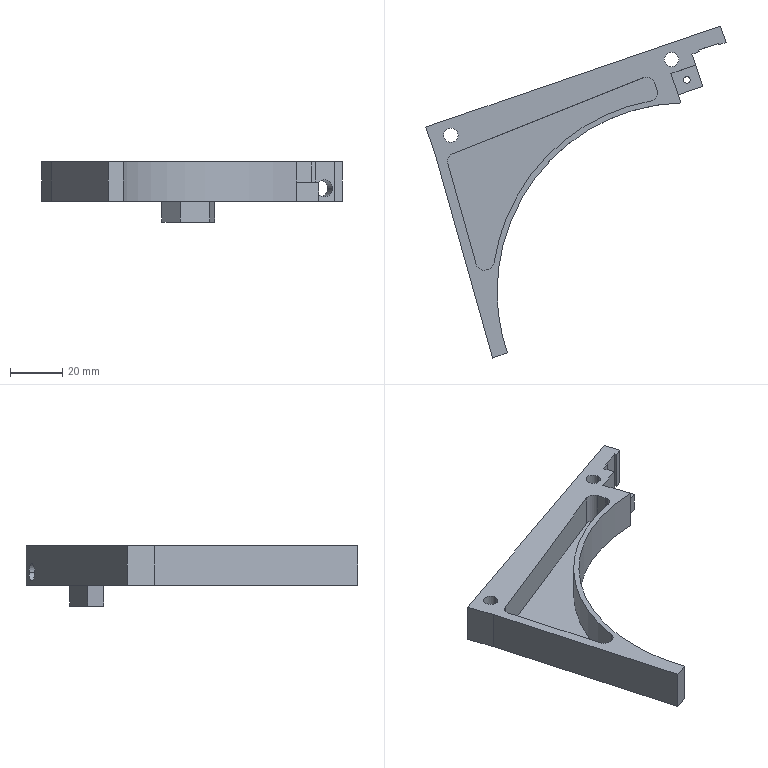Part | SolidWorks | features Cut 4, HoleWzd 2, Extrusion 1, ICE 1 | 1 solid | 45 faces | box 114.513 x 126.581 x 23 mm | volume 34516 mm3 | plane 28 | cylinder 17 | commonest cylinder face diameters 6 x6 5.5 x4 2.5 x2 6.5 x2 144 x2 148 x1
STEP:
#1=CARTESIAN_POINT('',(227.407,180.394,0.));
#2=VERTEX_POINT('',#1);
#3=CARTESIAN_POINT('',(229.907,180.394,0.));
#4=VERTEX_POINT('',#3);
#5=CARTESIAN_POINT('',(228.657,180.394,0.));
#6=DIRECTION('',(0.,0.,1.));
#7=DIRECTION('',(1.,0.,0.));
#8=AXIS2_PLACEMENT_3D('',#5,#6,#7);
#9=CIRCLE('',#8,1.25);
#10=EDGE_CURVE('',#2,#4,#9,.T.);
#11=ORIENTED_EDGE('',*,*,#10,.F.);
#12=CARTESIAN_POINT('',(227.407,180.394,7.));
#13=VERTEX_POINT('',#12);
#14=CARTESIAN_POINT('',(227.407,180.394,7.));
#15=DIRECTION('',(0.,0.,1.));
#16=VECTOR('',#15,1000.);
#17=LINE('',#14,#16);
#18=EDGE_CURVE('',#2,#13,#17,.T.);
#19=ORIENTED_EDGE('',*,*,#18,.T.);
#20=CARTESIAN_POINT('',(229.907,180.394,7.));
#21=VERTEX_POINT('',#20);
#22=CARTESIAN_POINT('',(228.657,180.394,7.));
#23=DIRECTION('',(0.,0.,1.));
#24=DIRECTION('',(1.,0.,0.));
#25=AXIS2_PLACEMENT_3D('',#22,#23,#24);
#26=CIRCLE('',#25,1.25);
#27=EDGE_CURVE('',#13,#21,#26,.T.);
#28=ORIENTED_EDGE('',*,*,#27,.T.);
#29=CARTESIAN_POINT('',(229.907,180.394,7.));
#30=DIRECTION('',(0.,0.,1.));
#31=VECTOR('',#30,1000.);
#32=LINE('',#29,#31);
#33=EDGE_CURVE('',#4,#21,#32,.T.);
#34=ORIENTED_EDGE('',*,*,#33,.F.);
#35=EDGE_LOOP('',(#11,#19,#28,#34));
#36=FACE_OUTER_BOUND('',#35,.T.);
#37=CARTESIAN_POINT('',(228.657,180.394,7.));
#38=DIRECTION('',(0.,0.,1.));
#39=DIRECTION('',(1.,0.,0.));
#40=AXIS2_PLACEMENT_3D('',#37,#38,#39);
#41=CYLINDRICAL_SURFACE('',#40,1.25);
#42=ADVANCED_FACE('',(#36),#41,.F.);
#43=CARTESIAN_POINT('',(238.03,199.762,5.));
#44=VERTEX_POINT('',#43);
#45=CARTESIAN_POINT('',(231.882,197.653,5.));
#46=VERTEX_POINT('',#45);
#47=CARTESIAN_POINT('',(234.956,198.708,5.));
#48=DIRECTION('',(-0.3245,0.9459,0.));
#49=DIRECTION('',(-0.9459,-0.3245,0.));
#50=AXIS2_PLACEMENT_3D('',#47,#48,#49);
#51=CIRCLE('',#50,3.25);
#52=EDGE_CURVE('',#44,#46,#51,.T.);
#53=ORIENTED_EDGE('',*,*,#52,.T.);
#54=CARTESIAN_POINT('',(233.829,191.978,5.));
#55=VERTEX_POINT('',#54);
#56=CARTESIAN_POINT('',(233.829,191.978,5.));
#57=DIRECTION('',(0.3245,-0.9459,0.));
#58=VECTOR('',#57,1000.);
#59=LINE('',#56,#58);
#60=EDGE_CURVE('',#46,#55,#59,.T.);
#61=ORIENTED_EDGE('',*,*,#60,.T.);
#62=CARTESIAN_POINT('',(239.977,194.087,5.));
#63=VERTEX_POINT('',#62);
#64=CARTESIAN_POINT('',(236.903,193.032,5.));
#65=DIRECTION('',(0.3245,-0.9459,0.));
#66=DIRECTION('',(0.9459,0.3245,0.));
#67=AXIS2_PLACEMENT_3D('',#64,#65,#66);
#68=CIRCLE('',#67,3.25);
#69=EDGE_CURVE('',#55,#63,#68,.T.);
#70=ORIENTED_EDGE('',*,*,#69,.T.);
#71=CARTESIAN_POINT('',(239.977,194.087,5.));
#72=DIRECTION('',(0.3245,-0.9459,0.));
#73=VECTOR('',#72,1000.);
#74=LINE('',#71,#73);
#75=EDGE_CURVE('',#44,#63,#74,.T.);
#76=ORIENTED_EDGE('',*,*,#75,.F.);
#77=EDGE_LOOP('',(#53,#61,#70,#76));
#78=FACE_OUTER_BOUND('',#77,.T.);
#79=CARTESIAN_POINT('',(236.903,193.032,5.));
#80=DIRECTION('',(0.3245,-0.9459,0.));
#81=DIRECTION('',(0.9459,0.3245,0.));
#82=AXIS2_PLACEMENT_3D('',#79,#80,#81);
#83=CYLINDRICAL_SURFACE('',#82,3.25);
#84=ADVANCED_FACE('',(#78),#83,.F.);
#85=CARTESIAN_POINT('',(220.059,188.197,0.));
#86=VERTEX_POINT('',#85);
#87=CARTESIAN_POINT('',(225.559,188.197,0.));
#88=VERTEX_POINT('',#87);
#89=CARTESIAN_POINT('',(222.809,188.197,0.));
#90=DIRECTION('',(0.,0.,1.));
#91=DIRECTION('',(1.,0.,0.));
#92=AXIS2_PLACEMENT_3D('',#89,#90,#91);
#93=CIRCLE('',#92,2.75);
#94=EDGE_CURVE('',#86,#88,#93,.T.);
#95=ORIENTED_EDGE('',*,*,#94,.F.);
#96=CARTESIAN_POINT('',(220.059,188.197,15.));
#97=VERTEX_POINT('',#96);
#98=CARTESIAN_POINT('',(220.059,188.197,-8.));
#99=DIRECTION('',(0.,0.,1.));
#100=VECTOR('',#99,1000.);
#101=LINE('',#98,#100);
#102=EDGE_CURVE('',#86,#97,#101,.T.);
#103=ORIENTED_EDGE('',*,*,#102,.T.);
#104=CARTESIAN_POINT('',(225.559,188.197,15.));
#105=VERTEX_POINT('',#104);
#106=CARTESIAN_POINT('',(222.809,188.197,15.));
#107=DIRECTION('',(0.,0.,1.));
#108=DIRECTION('',(-1.,0.,0.));
#109=AXIS2_PLACEMENT_3D('',#106,#107,#108);
#110=CIRCLE('',#109,2.75);
#111=EDGE_CURVE('',#97,#105,#110,.T.);
#112=ORIENTED_EDGE('',*,*,#111,.T.);
#113=CARTESIAN_POINT('',(225.559,188.197,-8.));
#114=DIRECTION('',(0.,0.,1.));
#115=VECTOR('',#114,1000.);
#116=LINE('',#113,#115);
#117=EDGE_CURVE('',#88,#105,#116,.T.);
#118=ORIENTED_EDGE('',*,*,#117,.F.);
#119=EDGE_LOOP('',(#95,#103,#112,#118));
#120=FACE_OUTER_BOUND('',#119,.T.);
#121=CARTESIAN_POINT('',(222.809,188.197,-8.));
#122=DIRECTION('',(0.,0.,1.));
#123=DIRECTION('',(1.,0.,0.));
#124=AXIS2_PLACEMENT_3D('',#121,#122,#123);
#125=CYLINDRICAL_SURFACE('',#124,2.75);
#126=ADVANCED_FACE('',(#120),#125,.F.);
#127=CARTESIAN_POINT('',(135.875,159.317,0.));
#128=VERTEX_POINT('',#127);
#129=CARTESIAN_POINT('',(141.375,159.317,0.));
#130=VERTEX_POINT('',#129);
#131=CARTESIAN_POINT('',(138.625,159.317,0.));
#132=DIRECTION('',(0.,0.,1.));
#133=DIRECTION('',(1.,0.,0.));
#134=AXIS2_PLACEMENT_3D('',#131,#132,#133);
#135=CIRCLE('',#134,2.75);
#136=EDGE_CURVE('',#128,#130,#135,.T.);
#137=ORIENTED_EDGE('',*,*,#136,.F.);
#138=CARTESIAN_POINT('',(135.875,159.317,15.));
#139=VERTEX_POINT('',#138);
#140=CARTESIAN_POINT('',(135.875,159.317,-8.));
#141=DIRECTION('',(0.,0.,1.));
#142=VECTOR('',#141,1000.);
#143=LINE('',#140,#142);
#144=EDGE_CURVE('',#128,#139,#143,.T.);
#145=ORIENTED_EDGE('',*,*,#144,.T.);
#146=CARTESIAN_POINT('',(141.375,159.317,15.));
#147=VERTEX_POINT('',#146);
#148=CARTESIAN_POINT('',(138.625,159.317,15.));
#149=DIRECTION('',(0.,0.,1.));
#150=DIRECTION('',(-1.,0.,0.));
#151=AXIS2_PLACEMENT_3D('',#148,#149,#150);
#152=CIRCLE('',#151,2.75);
#153=EDGE_CURVE('',#139,#147,#152,.T.);
#154=ORIENTED_EDGE('',*,*,#153,.T.);
#155=CARTESIAN_POINT('',(141.375,159.317,-8.));
#156=DIRECTION('',(0.,0.,1.));
#157=VECTOR('',#156,1000.);
#158=LINE('',#155,#157);
#159=EDGE_CURVE('',#130,#147,#158,.T.);
#160=ORIENTED_EDGE('',*,*,#159,.F.);
#161=EDGE_LOOP('',(#137,#145,#154,#160));
#162=FACE_OUTER_BOUND('',#161,.T.);
#163=CARTESIAN_POINT('',(138.625,159.317,-8.));
#164=DIRECTION('',(0.,0.,1.));
#165=DIRECTION('',(1.,0.,0.));
#166=AXIS2_PLACEMENT_3D('',#163,#164,#165);
#167=CYLINDRICAL_SURFACE('',#166,2.75);
#168=ADVANCED_FACE('',(#162),#167,.F.);
#169=CARTESIAN_POINT('',(217.46,175.388,3.));
#170=VERTEX_POINT('',#169);
#171=CARTESIAN_POINT('',(217.298,176.361,3.));
#172=VERTEX_POINT('',#171);
#173=CARTESIAN_POINT('',(214.46,175.388,3.));
#174=DIRECTION('',(0.,0.,1.));
#175=DIRECTION('',(-1.,0.,0.));
#176=AXIS2_PLACEMENT_3D('',#173,#174,#175);
#177=CIRCLE('',#176,3.);
#178=EDGE_CURVE('',#170,#172,#177,.T.);
#179=ORIENTED_EDGE('',*,*,#178,.F.);
#180=CARTESIAN_POINT('',(217.46,175.388,15.));
#181=VERTEX_POINT('',#180);
#182=CARTESIAN_POINT('',(217.46,175.388,3.));
#183=DIRECTION('',(0.,0.,1.));
#184=VECTOR('',#183,1000.);
#185=LINE('',#182,#184);
#186=EDGE_CURVE('',#170,#181,#185,.T.);
#187=ORIENTED_EDGE('',*,*,#186,.T.);
#188=CARTESIAN_POINT('',(217.298,176.361,15.));
#189=VERTEX_POINT('',#188);
#190=CARTESIAN_POINT('',(214.46,175.388,15.));
#191=DIRECTION('',(0.,0.,1.));
#192=DIRECTION('',(-1.,0.,0.));
#193=AXIS2_PLACEMENT_3D('',#190,#191,#192);
#194=CIRCLE('',#193,3.);
#195=EDGE_CURVE('',#181,#189,#194,.T.);
#196=ORIENTED_EDGE('',*,*,#195,.T.);
#197=CARTESIAN_POINT('',(217.298,176.361,3.));
#198=DIRECTION('',(0.,0.,1.));
#199=VECTOR('',#198,1000.);
#200=LINE('',#197,#199);
#201=EDGE_CURVE('',#172,#189,#200,.T.);
#202=ORIENTED_EDGE('',*,*,#201,.F.);
#203=EDGE_LOOP('',(#179,#187,#196,#202));
#204=FACE_OUTER_BOUND('',#203,.T.);
#205=CARTESIAN_POINT('',(214.46,175.388,3.));
#206=DIRECTION('',(0.,0.,1.));
#207=DIRECTION('',(1.,0.,0.));
#208=AXIS2_PLACEMENT_3D('',#205,#206,#207);
#209=CYLINDRICAL_SURFACE('',#208,3.);
#210=ADVANCED_FACE('',(#204),#209,.F.);
#211=CARTESIAN_POINT('',(226.383,171.615,15.));
#212=VERTEX_POINT('',#211);
#213=CARTESIAN_POINT('',(156.293,99.641,15.));
#214=VERTEX_POINT('',#213);
#215=CARTESIAN_POINT('',(228.293,99.641,15.));
#216=DIRECTION('',(0.,0.,1.));
#217=DIRECTION('',(1.,0.,0.));
#218=AXIS2_PLACEMENT_3D('',#215,#216,#217);
#219=CIRCLE('',#218,72.);
#220=EDGE_CURVE('',#212,#214,#219,.T.);
#221=ORIENTED_EDGE('',*,*,#220,.T.);
#222=CARTESIAN_POINT('',(156.293,99.641,0.));
#223=VERTEX_POINT('',#222);
#224=CARTESIAN_POINT('',(156.293,99.641,15.));
#225=DIRECTION('',(0.,0.,-1.));
#226=VECTOR('',#225,1000.);
#227=LINE('',#224,#226);
#228=EDGE_CURVE('',#214,#223,#227,.T.);
#229=ORIENTED_EDGE('',*,*,#228,.T.);
#230=CARTESIAN_POINT('',(226.383,171.615,0.));
#231=VERTEX_POINT('',#230);
#232=CARTESIAN_POINT('',(228.293,99.641,0.));
#233=DIRECTION('',(0.,0.,1.));
#234=DIRECTION('',(1.,0.,0.));
#235=AXIS2_PLACEMENT_3D('',#232,#233,#234);
#236=CIRCLE('',#235,72.);
#237=EDGE_CURVE('',#231,#223,#236,.T.);
#238=ORIENTED_EDGE('',*,*,#237,.F.);
#239=CARTESIAN_POINT('',(226.383,171.615,15.));
#240=DIRECTION('',(0.,0.,-1.));
#241=VECTOR('',#240,1000.);
#242=LINE('',#239,#241);
#243=EDGE_CURVE('',#212,#231,#242,.T.);
#244=ORIENTED_EDGE('',*,*,#243,.F.);
#245=EDGE_LOOP('',(#221,#229,#238,#244));
#246=FACE_OUTER_BOUND('',#245,.T.);
#247=CARTESIAN_POINT('',(228.293,99.641,15.));
#248=DIRECTION('',(0.,0.,-1.));
#249=DIRECTION('',(-1.,0.,0.));
#250=AXIS2_PLACEMENT_3D('',#247,#248,#249);
#251=CYLINDRICAL_SURFACE('',#250,72.);
#252=ADVANCED_FACE('',(#246),#251,.F.);
#253=CARTESIAN_POINT('',(234.772,177.966,7.));
#254=VERTEX_POINT('',#253);
#255=CARTESIAN_POINT('',(234.772,177.966,0.));
#256=VERTEX_POINT('',#255);
#257=CARTESIAN_POINT('',(234.772,177.966,15.));
#258=DIRECTION('',(0.,0.,-1.));
#259=VECTOR('',#258,1000.);
#260=LINE('',#257,#259);
#261=EDGE_CURVE('',#254,#256,#260,.T.);
#262=ORIENTED_EDGE('',*,*,#261,.F.);
#263=CARTESIAN_POINT('',(225.316,174.727,7.));
#264=VERTEX_POINT('',#263);
#265=CARTESIAN_POINT('',(234.772,177.966,7.));
#266=DIRECTION('',(0.946,0.324,0.));
#267=VECTOR('',#266,1000.);
#268=LINE('',#265,#267);
#269=EDGE_CURVE('',#264,#254,#268,.T.);
#270=ORIENTED_EDGE('',*,*,#269,.F.);
#271=CARTESIAN_POINT('',(225.316,174.727,0.));
#272=VERTEX_POINT('',#271);
#273=CARTESIAN_POINT('',(225.316,174.727,15.));
#274=DIRECTION('',(0.,0.,-1.));
#275=VECTOR('',#274,1000.);
#276=LINE('',#273,#275);
#277=EDGE_CURVE('',#264,#272,#276,.T.);
#278=ORIENTED_EDGE('',*,*,#277,.T.);
#279=CARTESIAN_POINT('',(234.772,177.966,0.));
#280=DIRECTION('',(-0.946,-0.324,0.));
#281=VECTOR('',#280,1000.);
#282=LINE('',#279,#281);
#283=EDGE_CURVE('',#256,#272,#282,.T.);
#284=ORIENTED_EDGE('',*,*,#283,.F.);
#285=EDGE_LOOP('',(#262,#270,#278,#284));
#286=FACE_OUTER_BOUND('',#285,.T.);
#287=CARTESIAN_POINT('',(234.772,177.966,15.));
#288=DIRECTION('',(0.324,-0.946,0.));
#289=DIRECTION('',(0.946,0.324,0.));
#290=AXIS2_PLACEMENT_3D('',#287,#288,#289);
#291=PLANE('',#290);
#292=ADVANCED_FACE('',(#286),#291,.T.);
#293=CARTESIAN_POINT('',(231.999,186.064,7.));
#294=VERTEX_POINT('',#293);
#295=CARTESIAN_POINT('',(234.772,177.966,7.));
#296=DIRECTION('',(-0.324,0.946,0.));
#297=VECTOR('',#296,1000.);
#298=LINE('',#295,#297);
#299=EDGE_CURVE('',#254,#294,#298,.T.);
#300=ORIENTED_EDGE('',*,*,#299,.F.);
#301=ORIENTED_EDGE('',*,*,#261,.T.);
#302=CARTESIAN_POINT('',(231.999,186.064,0.));
#303=VERTEX_POINT('',#302);
#304=CARTESIAN_POINT('',(234.772,177.966,0.));
#305=DIRECTION('',(-0.324,0.946,0.));
#306=VECTOR('',#305,1000.);
#307=LINE('',#304,#306);
#308=EDGE_CURVE('',#256,#303,#307,.T.);
#309=ORIENTED_EDGE('',*,*,#308,.T.);
#310=CARTESIAN_POINT('',(231.999,186.064,15.));
#311=DIRECTION('',(0.,0.,-1.));
#312=VECTOR('',#311,1000.);
#313=LINE('',#310,#312);
#314=EDGE_CURVE('',#294,#303,#313,.T.);
#315=ORIENTED_EDGE('',*,*,#314,.F.);
#316=EDGE_LOOP('',(#300,#301,#309,#315));
#317=FACE_OUTER_BOUND('',#316,.T.);
#318=CARTESIAN_POINT('',(234.772,177.966,15.));
#319=DIRECTION('',(-0.946,-0.324,0.));
#320=DIRECTION('',(0.324,-0.946,0.));
#321=AXIS2_PLACEMENT_3D('',#318,#319,#320);
#322=PLANE('',#321);
#323=ADVANCED_FACE('',(#317),#322,.F.);
#324=CARTESIAN_POINT('',(228.657,180.394,0.));
#325=DIRECTION('',(0.,0.,1.));
#326=DIRECTION('',(1.,0.,0.));
#327=AXIS2_PLACEMENT_3D('',#324,#325,#326);
#328=CIRCLE('',#327,1.25);
#329=EDGE_CURVE('',#4,#2,#328,.T.);
#330=ORIENTED_EDGE('',*,*,#329,.T.);
#331=ORIENTED_EDGE('',*,*,#10,.T.);
#332=EDGE_LOOP('',(#330,#331));
#333=FACE_BOUND('',#332,.T.);
#334=CARTESIAN_POINT('',(222.809,188.197,0.));
#335=DIRECTION('',(0.,0.,1.));
#336=DIRECTION('',(1.,0.,0.));
#337=AXIS2_PLACEMENT_3D('',#334,#335,#336);
#338=CIRCLE('',#337,2.75);
#339=EDGE_CURVE('',#88,#86,#338,.T.);
#340=ORIENTED_EDGE('',*,*,#339,.T.);
#341=ORIENTED_EDGE('',*,*,#94,.T.);
#342=EDGE_LOOP('',(#340,#341));
#343=FACE_BOUND('',#342,.T.);
#344=CARTESIAN_POINT('',(138.625,159.317,0.));
#345=DIRECTION('',(0.,0.,1.));
#346=DIRECTION('',(1.,0.,0.));
#347=AXIS2_PLACEMENT_3D('',#344,#345,#346);
#348=CIRCLE('',#347,2.75);
#349=EDGE_CURVE('',#130,#128,#348,.T.);
#350=ORIENTED_EDGE('',*,*,#349,.T.);
#351=ORIENTED_EDGE('',*,*,#136,.T.);
#352=EDGE_LOOP('',(#350,#351));
#353=FACE_BOUND('',#352,.T.);
#354=CARTESIAN_POINT('',(129.111,162.396,0.));
#355=VERTEX_POINT('',#354);
#356=CARTESIAN_POINT('',(132.681,151.992,0.));
#357=VERTEX_POINT('',#356);
#358=CARTESIAN_POINT('',(129.111,162.396,0.));
#359=DIRECTION('',(0.3245,-0.9459,0.));
#360=VECTOR('',#359,1000.);
#361=LINE('',#358,#360);
#362=EDGE_CURVE('',#355,#357,#361,.T.);
#363=ORIENTED_EDGE('',*,*,#362,.F.);
#364=CARTESIAN_POINT('',(241.482,200.947,0.));
#365=VERTEX_POINT('',#364);
#366=CARTESIAN_POINT('',(129.111,162.396,0.));
#367=DIRECTION('',(0.9459,0.3245,0.));
#368=VECTOR('',#367,1000.);
#369=LINE('',#366,#368);
#370=EDGE_CURVE('',#355,#365,#369,.T.);
#371=ORIENTED_EDGE('',*,*,#370,.T.);
#372=CARTESIAN_POINT('',(243.624,194.704,0.));
#373=VERTEX_POINT('',#372);
#374=CARTESIAN_POINT('',(241.482,200.947,0.));
#375=DIRECTION('',(0.3245,-0.9459,0.));
#376=VECTOR('',#375,1000.);
#377=LINE('',#374,#376);
#378=EDGE_CURVE('',#365,#373,#377,.T.);
#379=ORIENTED_EDGE('',*,*,#378,.T.);
#380=CARTESIAN_POINT('',(240.786,193.731,0.));
#381=VERTEX_POINT('',#380);
#382=CARTESIAN_POINT('',(243.624,194.704,0.));
#383=DIRECTION('',(-0.9459,-0.3245,0.));
#384=VECTOR('',#383,1000.);
#385=LINE('',#382,#384);
#386=EDGE_CURVE('',#373,#381,#385,.T.);
#387=ORIENTED_EDGE('',*,*,#386,.T.);
#388=CARTESIAN_POINT('',(240.592,194.298,0.));
#389=VERTEX_POINT('',#388);
#390=CARTESIAN_POINT('',(240.786,193.731,0.));
#391=DIRECTION('',(-0.3245,0.9459,0.));
#392=VECTOR('',#391,1000.);
#393=LINE('',#390,#392);
#394=EDGE_CURVE('',#381,#389,#393,.T.);
#395=ORIENTED_EDGE('',*,*,#394,.T.);
#396=CARTESIAN_POINT('',(233.214,191.767,0.));
#397=VERTEX_POINT('',#396);
#398=CARTESIAN_POINT('',(240.592,194.298,0.));
#399=DIRECTION('',(-0.9459,-0.3245,0.));
#400=VECTOR('',#399,1000.);
#401=LINE('',#398,#400);
#402=EDGE_CURVE('',#389,#397,#401,.T.);
#403=ORIENTED_EDGE('',*,*,#402,.T.);
#404=CARTESIAN_POINT('',(233.408,191.199,0.));
#405=VERTEX_POINT('',#404);
#406=CARTESIAN_POINT('',(233.214,191.767,0.));
#407=DIRECTION('',(0.3245,-0.9459,0.));
#408=VECTOR('',#407,1000.);
#409=LINE('',#406,#408);
#410=EDGE_CURVE('',#397,#405,#409,.T.);
#411=ORIENTED_EDGE('',*,*,#410,.T.);
#412=CARTESIAN_POINT('',(230.571,190.226,0.));
#413=VERTEX_POINT('',#412);
#414=CARTESIAN_POINT('',(230.571,190.226,0.));
#415=DIRECTION('',(0.9459,0.3245,0.));
#416=VECTOR('',#415,1000.);
#417=LINE('',#414,#416);
#418=EDGE_CURVE('',#413,#405,#417,.T.);
#419=ORIENTED_EDGE('',*,*,#418,.F.);
#420=CARTESIAN_POINT('',(231.999,186.064,0.));
#421=DIRECTION('',(-0.3245,0.9459,0.));
#422=VECTOR('',#421,1000.);
#423=LINE('',#420,#422);
#424=EDGE_CURVE('',#303,#413,#423,.T.);
#425=ORIENTED_EDGE('',*,*,#424,.F.);
#426=ORIENTED_EDGE('',*,*,#308,.F.);
#427=ORIENTED_EDGE('',*,*,#283,.T.);
#428=CARTESIAN_POINT('',(226.383,171.615,0.));
#429=DIRECTION('',(-0.3245,0.9459,0.));
#430=VECTOR('',#429,1000.);
#431=LINE('',#428,#430);
#432=EDGE_CURVE('',#231,#272,#431,.T.);
#433=ORIENTED_EDGE('',*,*,#432,.F.);
#434=ORIENTED_EDGE('',*,*,#237,.T.);
#435=CARTESIAN_POINT('',(160.178,76.31,0.));
#436=VERTEX_POINT('',#435);
#437=CARTESIAN_POINT('',(228.293,99.641,0.));
#438=DIRECTION('',(0.,0.,1.));
#439=DIRECTION('',(1.,0.,0.));
#440=AXIS2_PLACEMENT_3D('',#437,#438,#439);
#441=CIRCLE('',#440,72.);
#442=EDGE_CURVE('',#223,#436,#441,.T.);
#443=ORIENTED_EDGE('',*,*,#442,.T.);
#444=CARTESIAN_POINT('',(154.501,74.366,0.));
#445=VERTEX_POINT('',#444);
#446=CARTESIAN_POINT('',(154.501,74.366,0.));
#447=DIRECTION('',(0.946,0.324,0.));
#448=VECTOR('',#447,1000.);
#449=LINE('',#446,#448);
#450=EDGE_CURVE('',#445,#436,#449,.T.);
#451=ORIENTED_EDGE('',*,*,#450,.F.);
#452=CARTESIAN_POINT('',(132.681,151.992,0.));
#453=DIRECTION('',(0.2706,-0.9627,0.));
#454=VECTOR('',#453,1000.);
#455=LINE('',#452,#454);
#456=EDGE_CURVE('',#357,#445,#455,.T.);
#457=ORIENTED_EDGE('',*,*,#456,.F.);
#458=EDGE_LOOP('',(#363,#371,#379,#387,#395,#403,#411,#419,#425,#426,#427,#433,#434,#443,#451,#457));
#459=FACE_OUTER_BOUND('',#458,.T.);
#460=CARTESIAN_POINT('',(194.997,184.333,0.));
#461=VERTEX_POINT('',#460);
#462=CARTESIAN_POINT('',(193.224,175.267,0.));
#463=VERTEX_POINT('',#462);
#464=CARTESIAN_POINT('',(194.997,184.333,0.));
#465=DIRECTION('',(-0.1919,-0.9814,0.));
#466=VECTOR('',#465,1000.);
#467=LINE('',#464,#466);
#468=EDGE_CURVE('',#461,#463,#467,.T.);
#469=ORIENTED_EDGE('',*,*,#468,.F.);
#470=CARTESIAN_POINT('',(174.909,177.441,0.));
#471=VERTEX_POINT('',#470);
#472=CARTESIAN_POINT('',(174.909,177.441,0.));
#473=DIRECTION('',(0.9459,0.3245,0.));
#474=VECTOR('',#473,1000.);
#475=LINE('',#472,#474);
#476=EDGE_CURVE('',#471,#461,#475,.T.);
#477=ORIENTED_EDGE('',*,*,#476,.F.);
#478=CARTESIAN_POINT('',(181.874,171.373,0.));
#479=VERTEX_POINT('',#478);
#480=CARTESIAN_POINT('',(181.874,171.373,0.));
#481=DIRECTION('',(-0.754,0.6569,0.));
#482=VECTOR('',#481,1000.);
#483=LINE('',#480,#482);
#484=EDGE_CURVE('',#479,#471,#483,.T.);
#485=ORIENTED_EDGE('',*,*,#484,.F.);
#486=CARTESIAN_POINT('',(181.874,171.373,0.));
#487=DIRECTION('',(-0.9459,-0.3245,0.));
#488=VECTOR('',#487,1000.);
#489=LINE('',#486,#488);
#490=EDGE_CURVE('',#463,#479,#489,.T.);
#491=ORIENTED_EDGE('',*,*,#490,.F.);
#492=EDGE_LOOP('',(#469,#477,#485,#491));
#493=FACE_BOUND('',#492,.T.);
#494=CARTESIAN_POINT('',(228.293,99.641,0.));
#495=DIRECTION('',(0.,0.,1.));
#496=DIRECTION('',(1.,0.,0.));
#497=AXIS2_PLACEMENT_3D('',#494,#495,#496);
#498=PLANE('',#497);
#499=ADVANCED_FACE('',(#333,#343,#353,#459,#493),#498,.F.);
#500=ORIENTED_EDGE('',*,*,#362,.T.);
#501=CARTESIAN_POINT('',(132.681,151.992,15.));
#502=VERTEX_POINT('',#501);
#503=CARTESIAN_POINT('',(132.681,151.992,15.));
#504=DIRECTION('',(0.,0.,-1.));
#505=VECTOR('',#504,1000.);
#506=LINE('',#503,#505);
#507=EDGE_CURVE('',#502,#357,#506,.T.);
#508=ORIENTED_EDGE('',*,*,#507,.F.);
#509=CARTESIAN_POINT('',(129.111,162.396,15.));
#510=VERTEX_POINT('',#509);
#511=CARTESIAN_POINT('',(129.111,162.396,15.));
#512=DIRECTION('',(0.3245,-0.9459,0.));
#513=VECTOR('',#512,1000.);
#514=LINE('',#511,#513);
#515=EDGE_CURVE('',#510,#502,#514,.T.);
#516=ORIENTED_EDGE('',*,*,#515,.F.);
#517=CARTESIAN_POINT('',(129.111,162.396,15.));
#518=DIRECTION('',(0.,0.,-1.));
#519=VECTOR('',#518,1000.);
#520=LINE('',#517,#519);
#521=EDGE_CURVE('',#510,#355,#520,.T.);
#522=ORIENTED_EDGE('',*,*,#521,.T.);
#523=EDGE_LOOP('',(#500,#508,#516,#522));
#524=FACE_OUTER_BOUND('',#523,.T.);
#525=CARTESIAN_POINT('',(129.111,162.396,15.));
#526=DIRECTION('',(0.9459,0.3245,0.));
#527=DIRECTION('',(-0.3245,0.9459,0.));
#528=AXIS2_PLACEMENT_3D('',#525,#526,#527);
#529=PLANE('',#528);
#530=ADVANCED_FACE('',(#524),#529,.F.);
#531=ORIENTED_EDGE('',*,*,#456,.T.);
#532=CARTESIAN_POINT('',(154.501,74.366,15.));
#533=VERTEX_POINT('',#532);
#534=CARTESIAN_POINT('',(154.501,74.366,15.));
#535=DIRECTION('',(0.,0.,-1.));
#536=VECTOR('',#535,1000.);
#537=LINE('',#534,#536);
#538=EDGE_CURVE('',#533,#445,#537,.T.);
#539=ORIENTED_EDGE('',*,*,#538,.F.);
#540=CARTESIAN_POINT('',(132.681,151.992,15.));
#541=DIRECTION('',(0.2706,-0.9627,0.));
#542=VECTOR('',#541,1000.);
#543=LINE('',#540,#542);
#544=EDGE_CURVE('',#502,#533,#543,.T.);
#545=ORIENTED_EDGE('',*,*,#544,.F.);
#546=ORIENTED_EDGE('',*,*,#507,.T.);
#547=EDGE_LOOP('',(#531,#539,#545,#546));
#548=FACE_OUTER_BOUND('',#547,.T.);
#549=CARTESIAN_POINT('',(132.681,151.992,15.));
#550=DIRECTION('',(0.9627,0.2706,0.));
#551=DIRECTION('',(-0.2706,0.9627,0.));
#552=AXIS2_PLACEMENT_3D('',#549,#550,#551);
#553=PLANE('',#552);
#554=ADVANCED_FACE('',(#548),#553,.F.);
#555=ORIENTED_EDGE('',*,*,#450,.T.);
#556=CARTESIAN_POINT('',(160.178,76.31,15.));
#557=VERTEX_POINT('',#556);
#558=CARTESIAN_POINT('',(160.178,76.31,15.));
#559=DIRECTION('',(0.,0.,-1.));
#560=VECTOR('',#559,1000.);
#561=LINE('',#558,#560);
#562=EDGE_CURVE('',#557,#436,#561,.T.);
#563=ORIENTED_EDGE('',*,*,#562,.F.);
#564=CARTESIAN_POINT('',(154.501,74.366,15.));
#565=DIRECTION('',(0.946,0.324,0.));
#566=VECTOR('',#565,1000.);
#567=LINE('',#564,#566);
#568=EDGE_CURVE('',#533,#557,#567,.T.);
#569=ORIENTED_EDGE('',*,*,#568,.F.);
#570=ORIENTED_EDGE('',*,*,#538,.T.);
#571=EDGE_LOOP('',(#555,#563,#569,#570));
#572=FACE_OUTER_BOUND('',#571,.T.);
#573=CARTESIAN_POINT('',(154.501,74.366,15.));
#574=DIRECTION('',(-0.324,0.946,0.));
#575=DIRECTION('',(-0.946,-0.324,0.));
#576=AXIS2_PLACEMENT_3D('',#573,#574,#575);
#577=PLANE('',#576);
#578=ADVANCED_FACE('',(#572),#577,.F.);
#579=ORIENTED_EDGE('',*,*,#228,.F.);
#580=CARTESIAN_POINT('',(228.293,99.641,15.));
#581=DIRECTION('',(0.,0.,1.));
#582=DIRECTION('',(1.,0.,0.));
#583=AXIS2_PLACEMENT_3D('',#580,#581,#582);
#584=CIRCLE('',#583,72.);
#585=EDGE_CURVE('',#214,#557,#584,.T.);
#586=ORIENTED_EDGE('',*,*,#585,.T.);
#587=ORIENTED_EDGE('',*,*,#562,.T.);
#588=ORIENTED_EDGE('',*,*,#442,.F.);
#589=EDGE_LOOP('',(#579,#586,#587,#588));
#590=FACE_OUTER_BOUND('',#589,.T.);
#591=CARTESIAN_POINT('',(228.293,99.641,15.));
#592=DIRECTION('',(0.,0.,-1.));
#593=DIRECTION('',(-1.,0.,0.));
#594=AXIS2_PLACEMENT_3D('',#591,#592,#593);
#595=CYLINDRICAL_SURFACE('',#594,72.);
#596=ADVANCED_FACE('',(#590),#595,.F.);
#597=ORIENTED_EDGE('',*,*,#432,.T.);
#598=ORIENTED_EDGE('',*,*,#277,.F.);
#599=CARTESIAN_POINT('',(222.54,182.819,7.));
#600=VERTEX_POINT('',#599);
#601=CARTESIAN_POINT('',(225.316,174.727,7.));
#602=DIRECTION('',(0.3245,-0.9459,0.));
#603=VECTOR('',#602,1000.);
#604=LINE('',#601,#603);
#605=EDGE_CURVE('',#600,#264,#604,.T.);
#606=ORIENTED_EDGE('',*,*,#605,.F.);
#607=CARTESIAN_POINT('',(222.54,182.819,15.));
#608=VERTEX_POINT('',#607);
#609=CARTESIAN_POINT('',(222.54,182.819,7.));
#610=DIRECTION('',(0.,0.,1.));
#611=VECTOR('',#610,1000.);
#612=LINE('',#609,#611);
#613=EDGE_CURVE('',#600,#608,#612,.T.);
#614=ORIENTED_EDGE('',*,*,#613,.T.);
#615=CARTESIAN_POINT('',(226.383,171.615,15.));
#616=DIRECTION('',(-0.3245,0.9459,0.));
#617=VECTOR('',#616,1000.);
#618=LINE('',#615,#617);
#619=EDGE_CURVE('',#212,#608,#618,.T.);
#620=ORIENTED_EDGE('',*,*,#619,.F.);
#621=ORIENTED_EDGE('',*,*,#243,.T.);
#622=EDGE_LOOP('',(#597,#598,#606,#614,#620,#621));
#623=FACE_OUTER_BOUND('',#622,.T.);
#624=CARTESIAN_POINT('',(226.383,171.615,15.));
#625=DIRECTION('',(-0.9459,-0.3245,0.));
#626=DIRECTION('',(0.3245,-0.9459,0.));
#627=AXIS2_PLACEMENT_3D('',#624,#625,#626);
#628=PLANE('',#627);
#629=ADVANCED_FACE('',(#623),#628,.F.);
#630=ORIENTED_EDGE('',*,*,#424,.T.);
#631=CARTESIAN_POINT('',(230.571,190.226,15.));
#632=VERTEX_POINT('',#631);
#633=CARTESIAN_POINT('',(230.571,190.226,15.));
#634=DIRECTION('',(0.,0.,-1.));
#635=VECTOR('',#634,1000.);
#636=LINE('',#633,#635);
#637=EDGE_CURVE('',#632,#413,#636,.T.);
#638=ORIENTED_EDGE('',*,*,#637,.F.);
#639=CARTESIAN_POINT('',(231.999,186.064,15.));
#640=VERTEX_POINT('',#639);
#641=CARTESIAN_POINT('',(231.999,186.064,15.));
#642=DIRECTION('',(-0.3245,0.9459,0.));
#643=VECTOR('',#642,1000.);
#644=LINE('',#641,#643);
#645=EDGE_CURVE('',#640,#632,#644,.T.);
#646=ORIENTED_EDGE('',*,*,#645,.F.);
#647=CARTESIAN_POINT('',(231.999,186.064,15.));
#648=DIRECTION('',(0.,0.,-1.));
#649=VECTOR('',#648,1000.);
#650=LINE('',#647,#649);
#651=EDGE_CURVE('',#640,#294,#650,.T.);
#652=ORIENTED_EDGE('',*,*,#651,.T.);
#653=ORIENTED_EDGE('',*,*,#314,.T.);
#654=EDGE_LOOP('',(#630,#638,#646,#652,#653));
#655=FACE_OUTER_BOUND('',#654,.T.);
#656=CARTESIAN_POINT('',(231.999,186.064,15.));
#657=DIRECTION('',(-0.9459,-0.3245,0.));
#658=DIRECTION('',(0.3245,-0.9459,0.));
#659=AXIS2_PLACEMENT_3D('',#656,#657,#658);
#660=PLANE('',#659);
#661=ADVANCED_FACE('',(#655),#660,.F.);
#662=ORIENTED_EDGE('',*,*,#418,.T.);
#663=CARTESIAN_POINT('',(233.408,191.199,15.));
#664=VERTEX_POINT('',#663);
#665=CARTESIAN_POINT('',(233.408,191.199,15.));
#666=DIRECTION('',(0.,0.,-1.));
#667=VECTOR('',#666,1000.);
#668=LINE('',#665,#667);
#669=EDGE_CURVE('',#664,#405,#668,.T.);
#670=ORIENTED_EDGE('',*,*,#669,.F.);
#671=CARTESIAN_POINT('',(230.571,190.226,15.));
#672=DIRECTION('',(0.9459,0.3245,0.));
#673=VECTOR('',#672,1000.);
#674=LINE('',#671,#673);
#675=EDGE_CURVE('',#632,#664,#674,.T.);
#676=ORIENTED_EDGE('',*,*,#675,.F.);
#677=ORIENTED_EDGE('',*,*,#637,.T.);
#678=EDGE_LOOP('',(#662,#670,#676,#677));
#679=FACE_OUTER_BOUND('',#678,.T.);
#680=CARTESIAN_POINT('',(230.571,190.226,15.));
#681=DIRECTION('',(-0.3245,0.9459,0.));
#682=DIRECTION('',(-0.9459,-0.3245,0.));
#683=AXIS2_PLACEMENT_3D('',#680,#681,#682);
#684=PLANE('',#683);
#685=ADVANCED_FACE('',(#679),#684,.F.);
#686=ORIENTED_EDGE('',*,*,#410,.F.);
#687=CARTESIAN_POINT('',(233.214,191.767,15.));
#688=VERTEX_POINT('',#687);
#689=CARTESIAN_POINT('',(233.214,191.767,15.));
#690=DIRECTION('',(0.,0.,-1.));
#691=VECTOR('',#690,1000.);
#692=LINE('',#689,#691);
#693=EDGE_CURVE('',#688,#397,#692,.T.);
#694=ORIENTED_EDGE('',*,*,#693,.F.);
#695=CARTESIAN_POINT('',(233.214,191.767,15.));
#696=DIRECTION('',(0.3245,-0.9459,0.));
#697=VECTOR('',#696,1000.);
#698=LINE('',#695,#697);
#699=EDGE_CURVE('',#688,#664,#698,.T.);
#700=ORIENTED_EDGE('',*,*,#699,.T.);
#701=ORIENTED_EDGE('',*,*,#669,.T.);
#702=EDGE_LOOP('',(#686,#694,#700,#701));
#703=FACE_OUTER_BOUND('',#702,.T.);
#704=CARTESIAN_POINT('',(233.214,191.767,15.));
#705=DIRECTION('',(0.9459,0.3245,0.));
#706=DIRECTION('',(-0.3245,0.9459,0.));
#707=AXIS2_PLACEMENT_3D('',#704,#705,#706);
#708=PLANE('',#707);
#709=ADVANCED_FACE('',(#703),#708,.T.);
#710=CARTESIAN_POINT('',(236.903,193.032,5.));
#711=DIRECTION('',(0.3245,-0.9459,0.));
#712=DIRECTION('',(0.9459,0.3245,0.));
#713=AXIS2_PLACEMENT_3D('',#710,#711,#712);
#714=CIRCLE('',#713,3.25);
#715=EDGE_CURVE('',#63,#55,#714,.T.);
#716=ORIENTED_EDGE('',*,*,#715,.F.);
#717=ORIENTED_EDGE('',*,*,#69,.F.);
#718=EDGE_LOOP('',(#716,#717));
#719=FACE_BOUND('',#718,.T.);
#720=ORIENTED_EDGE('',*,*,#402,.F.);
#721=CARTESIAN_POINT('',(240.592,194.298,15.));
#722=VERTEX_POINT('',#721);
#723=CARTESIAN_POINT('',(240.592,194.298,15.));
#724=DIRECTION('',(0.,0.,-1.));
#725=VECTOR('',#724,1000.);
#726=LINE('',#723,#725);
#727=EDGE_CURVE('',#722,#389,#726,.T.);
#728=ORIENTED_EDGE('',*,*,#727,.F.);
#729=CARTESIAN_POINT('',(240.592,194.298,15.));
#730=DIRECTION('',(-0.9459,-0.3245,0.));
#731=VECTOR('',#730,1000.);
#732=LINE('',#729,#731);
#733=EDGE_CURVE('',#722,#688,#732,.T.);
#734=ORIENTED_EDGE('',*,*,#733,.T.);
#735=ORIENTED_EDGE('',*,*,#693,.T.);
#736=EDGE_LOOP('',(#720,#728,#734,#735));
#737=FACE_OUTER_BOUND('',#736,.T.);
#738=CARTESIAN_POINT('',(240.592,194.298,15.));
#739=DIRECTION('',(0.3245,-0.9459,0.));
#740=DIRECTION('',(0.9459,0.3245,0.));
#741=AXIS2_PLACEMENT_3D('',#738,#739,#740);
#742=PLANE('',#741);
#743=ADVANCED_FACE('',(#719,#737),#742,.T.);
#744=ORIENTED_EDGE('',*,*,#394,.F.);
#745=CARTESIAN_POINT('',(240.786,193.731,15.));
#746=VERTEX_POINT('',#745);
#747=CARTESIAN_POINT('',(240.786,193.731,15.));
#748=DIRECTION('',(0.,0.,-1.));
#749=VECTOR('',#748,1000.);
#750=LINE('',#747,#749);
#751=EDGE_CURVE('',#746,#381,#750,.T.);
#752=ORIENTED_EDGE('',*,*,#751,.F.);
#753=CARTESIAN_POINT('',(240.786,193.731,15.));
#754=DIRECTION('',(-0.3245,0.9459,0.));
#755=VECTOR('',#754,1000.);
#756=LINE('',#753,#755);
#757=EDGE_CURVE('',#746,#722,#756,.T.);
#758=ORIENTED_EDGE('',*,*,#757,.T.);
#759=ORIENTED_EDGE('',*,*,#727,.T.);
#760=EDGE_LOOP('',(#744,#752,#758,#759));
#761=FACE_OUTER_BOUND('',#760,.T.);
#762=CARTESIAN_POINT('',(240.786,193.731,15.));
#763=DIRECTION('',(-0.9459,-0.3245,0.));
#764=DIRECTION('',(0.3245,-0.9459,0.));
#765=AXIS2_PLACEMENT_3D('',#762,#763,#764);
#766=PLANE('',#765);
#767=ADVANCED_FACE('',(#761),#766,.T.);
#768=ORIENTED_EDGE('',*,*,#386,.F.);
#769=CARTESIAN_POINT('',(243.624,194.704,15.));
#770=VERTEX_POINT('',#769);
#771=CARTESIAN_POINT('',(243.624,194.704,15.));
#772=DIRECTION('',(0.,0.,-1.));
#773=VECTOR('',#772,1000.);
#774=LINE('',#771,#773);
#775=EDGE_CURVE('',#770,#373,#774,.T.);
#776=ORIENTED_EDGE('',*,*,#775,.F.);
#777=CARTESIAN_POINT('',(243.624,194.704,15.));
#778=DIRECTION('',(-0.9459,-0.3245,0.));
#779=VECTOR('',#778,1000.);
#780=LINE('',#777,#779);
#781=EDGE_CURVE('',#770,#746,#780,.T.);
#782=ORIENTED_EDGE('',*,*,#781,.T.);
#783=ORIENTED_EDGE('',*,*,#751,.T.);
#784=EDGE_LOOP('',(#768,#776,#782,#783));
#785=FACE_OUTER_BOUND('',#784,.T.);
#786=CARTESIAN_POINT('',(243.624,194.704,15.));
#787=DIRECTION('',(0.3245,-0.9459,0.));
#788=DIRECTION('',(0.9459,0.3245,0.));
#789=AXIS2_PLACEMENT_3D('',#786,#787,#788);
#790=PLANE('',#789);
#791=ADVANCED_FACE('',(#785),#790,.T.);
#792=ORIENTED_EDGE('',*,*,#378,.F.);
#793=CARTESIAN_POINT('',(241.482,200.947,15.));
#794=VERTEX_POINT('',#793);
#795=CARTESIAN_POINT('',(241.482,200.947,15.));
#796=DIRECTION('',(0.,0.,-1.));
#797=VECTOR('',#796,1000.);
#798=LINE('',#795,#797);
#799=EDGE_CURVE('',#794,#365,#798,.T.);
#800=ORIENTED_EDGE('',*,*,#799,.F.);
#801=CARTESIAN_POINT('',(241.482,200.947,15.));
#802=DIRECTION('',(0.3245,-0.9459,0.));
#803=VECTOR('',#802,1000.);
#804=LINE('',#801,#803);
#805=EDGE_CURVE('',#794,#770,#804,.T.);
#806=ORIENTED_EDGE('',*,*,#805,.T.);
#807=ORIENTED_EDGE('',*,*,#775,.T.);
#808=EDGE_LOOP('',(#792,#800,#806,#807));
#809=FACE_OUTER_BOUND('',#808,.T.);
#810=CARTESIAN_POINT('',(241.482,200.947,15.));
#811=DIRECTION('',(0.9459,0.3245,0.));
#812=DIRECTION('',(-0.3245,0.9459,0.));
#813=AXIS2_PLACEMENT_3D('',#810,#811,#812);
#814=PLANE('',#813);
#815=ADVANCED_FACE('',(#809),#814,.T.);
#816=ORIENTED_EDGE('',*,*,#52,.F.);
#817=CARTESIAN_POINT('',(234.956,198.708,5.));
#818=DIRECTION('',(-0.3245,0.9459,0.));
#819=DIRECTION('',(-0.9459,-0.3245,0.));
#820=AXIS2_PLACEMENT_3D('',#817,#818,#819);
#821=CIRCLE('',#820,3.25);
#822=EDGE_CURVE('',#46,#44,#821,.T.);
#823=ORIENTED_EDGE('',*,*,#822,.F.);
#824=EDGE_LOOP('',(#816,#823));
#825=FACE_BOUND('',#824,.T.);
#826=ORIENTED_EDGE('',*,*,#370,.F.);
#827=ORIENTED_EDGE('',*,*,#521,.F.);
#828=CARTESIAN_POINT('',(129.111,162.396,15.));
#829=DIRECTION('',(0.9459,0.3245,0.));
#830=VECTOR('',#829,1000.);
#831=LINE('',#828,#830);
#832=EDGE_CURVE('',#510,#794,#831,.T.);
#833=ORIENTED_EDGE('',*,*,#832,.T.);
#834=ORIENTED_EDGE('',*,*,#799,.T.);
#835=EDGE_LOOP('',(#826,#827,#833,#834));
#836=FACE_OUTER_BOUND('',#835,.T.);
#837=CARTESIAN_POINT('',(129.111,162.396,15.));
#838=DIRECTION('',(-0.3245,0.9459,0.));
#839=DIRECTION('',(-0.9459,-0.3245,0.));
#840=AXIS2_PLACEMENT_3D('',#837,#838,#839);
#841=PLANE('',#840);
#842=ADVANCED_FACE('',(#825,#836),#841,.T.);
#843=CARTESIAN_POINT('',(222.809,188.197,15.));
#844=DIRECTION('',(0.,0.,1.));
#845=DIRECTION('',(-1.,0.,0.));
#846=AXIS2_PLACEMENT_3D('',#843,#844,#845);
#847=CIRCLE('',#846,2.75);
#848=EDGE_CURVE('',#105,#97,#847,.T.);
#849=ORIENTED_EDGE('',*,*,#848,.F.);
#850=ORIENTED_EDGE('',*,*,#111,.F.);
#851=EDGE_LOOP('',(#849,#850));
#852=FACE_BOUND('',#851,.T.);
#853=CARTESIAN_POINT('',(138.625,159.317,15.));
#854=DIRECTION('',(0.,0.,1.));
#855=DIRECTION('',(-1.,0.,0.));
#856=AXIS2_PLACEMENT_3D('',#853,#854,#855);
#857=CIRCLE('',#856,2.75);
#858=EDGE_CURVE('',#147,#139,#857,.T.);
#859=ORIENTED_EDGE('',*,*,#858,.F.);
#860=ORIENTED_EDGE('',*,*,#153,.F.);
#861=EDGE_LOOP('',(#859,#860));
#862=FACE_BOUND('',#861,.T.);
#863=ORIENTED_EDGE('',*,*,#619,.T.);
#864=CARTESIAN_POINT('',(222.54,182.819,15.));
#865=DIRECTION('',(-0.9459,-0.3245,0.));
#866=VECTOR('',#865,1000.);
#867=LINE('',#864,#866);
#868=EDGE_CURVE('',#640,#608,#867,.T.);
#869=ORIENTED_EDGE('',*,*,#868,.F.);
#870=ORIENTED_EDGE('',*,*,#645,.T.);
#871=ORIENTED_EDGE('',*,*,#675,.T.);
#872=ORIENTED_EDGE('',*,*,#699,.F.);
#873=ORIENTED_EDGE('',*,*,#733,.F.);
#874=ORIENTED_EDGE('',*,*,#757,.F.);
#875=ORIENTED_EDGE('',*,*,#781,.F.);
#876=ORIENTED_EDGE('',*,*,#805,.F.);
#877=ORIENTED_EDGE('',*,*,#832,.F.);
#878=ORIENTED_EDGE('',*,*,#515,.T.);
#879=ORIENTED_EDGE('',*,*,#544,.T.);
#880=ORIENTED_EDGE('',*,*,#568,.T.);
#881=ORIENTED_EDGE('',*,*,#585,.F.);
#882=ORIENTED_EDGE('',*,*,#220,.F.);
#883=EDGE_LOOP('',(#863,#869,#870,#871,#872,#873,#874,#875,#876,#877,#878,#879,#880,#881,#882));
#884=FACE_OUTER_BOUND('',#883,.T.);
#885=CARTESIAN_POINT('',(139.266,152.159,15.));
#886=VERTEX_POINT('',#885);
#887=CARTESIAN_POINT('',(137.489,148.561,15.));
#888=VERTEX_POINT('',#887);
#889=CARTESIAN_POINT('',(140.377,149.372,15.));
#890=DIRECTION('',(0.,0.,1.));
#891=DIRECTION('',(-1.,0.,0.));
#892=AXIS2_PLACEMENT_3D('',#889,#890,#891);
#893=CIRCLE('',#892,3.);
#894=EDGE_CURVE('',#886,#888,#893,.T.);
#895=ORIENTED_EDGE('',*,*,#894,.F.);
#896=CARTESIAN_POINT('',(212.285,181.276,15.));
#897=VERTEX_POINT('',#896);
#898=CARTESIAN_POINT('',(212.285,181.276,15.));
#899=DIRECTION('',(-0.9289,-0.3704,0.));
#900=VECTOR('',#899,1000.);
#901=LINE('',#898,#900);
#902=EDGE_CURVE('',#897,#886,#901,.T.);
#903=ORIENTED_EDGE('',*,*,#902,.F.);
#904=CARTESIAN_POINT('',(216.234,179.463,15.));
#905=VERTEX_POINT('',#904);
#906=CARTESIAN_POINT('',(213.396,178.489,15.));
#907=DIRECTION('',(0.,0.,1.));
#908=DIRECTION('',(-1.,0.,0.));
#909=AXIS2_PLACEMENT_3D('',#906,#907,#908);
#910=CIRCLE('',#909,3.);
#911=EDGE_CURVE('',#905,#897,#910,.T.);
#912=ORIENTED_EDGE('',*,*,#911,.F.);
#913=CARTESIAN_POINT('',(217.298,176.361,15.));
#914=DIRECTION('',(-0.3245,0.9459,0.));
#915=VECTOR('',#914,1000.);
#916=LINE('',#913,#915);
#917=EDGE_CURVE('',#189,#905,#916,.T.);
#918=ORIENTED_EDGE('',*,*,#917,.F.);
#919=ORIENTED_EDGE('',*,*,#195,.F.);
#920=CARTESIAN_POINT('',(214.999,172.437,15.));
#921=VERTEX_POINT('',#920);
#922=CARTESIAN_POINT('',(214.46,175.388,15.));
#923=DIRECTION('',(0.,0.,1.));
#924=DIRECTION('',(-1.,0.,0.));
#925=AXIS2_PLACEMENT_3D('',#922,#923,#924);
#926=CIRCLE('',#925,3.);
#927=EDGE_CURVE('',#921,#181,#926,.T.);
#928=ORIENTED_EDGE('',*,*,#927,.F.);
#929=CARTESIAN_POINT('',(155.118,110.657,15.));
#930=VERTEX_POINT('',#929);
#931=CARTESIAN_POINT('',(228.293,99.641,15.));
#932=DIRECTION('',(0.,0.,-1.));
#933=DIRECTION('',(-1.,0.,0.));
#934=AXIS2_PLACEMENT_3D('',#931,#932,#933);
#935=CIRCLE('',#934,74.);
#936=EDGE_CURVE('',#930,#921,#935,.T.);
#937=ORIENTED_EDGE('',*,*,#936,.F.);
#938=CARTESIAN_POINT('',(153.125,108.266,15.));
#939=VERTEX_POINT('',#938);
#940=CARTESIAN_POINT('',(152.151,111.104,15.));
#941=DIRECTION('',(0.,0.,1.));
#942=DIRECTION('',(-1.,0.,0.));
#943=AXIS2_PLACEMENT_3D('',#940,#941,#942);
#944=CIRCLE('',#943,3.);
#945=EDGE_CURVE('',#939,#930,#944,.T.);
#946=ORIENTED_EDGE('',*,*,#945,.F.);
#947=CARTESIAN_POINT('',(152.197,107.948,15.));
#948=VERTEX_POINT('',#947);
#949=CARTESIAN_POINT('',(153.125,108.266,15.));
#950=DIRECTION('',(0.9459,0.3245,0.));
#951=VECTOR('',#950,1000.);
#952=LINE('',#949,#951);
#953=EDGE_CURVE('',#948,#939,#952,.T.);
#954=ORIENTED_EDGE('',*,*,#953,.F.);
#955=CARTESIAN_POINT('',(148.336,109.974,15.));
#956=VERTEX_POINT('',#955);
#957=CARTESIAN_POINT('',(151.224,110.786,15.));
#958=DIRECTION('',(0.,0.,1.));
#959=DIRECTION('',(-1.,0.,0.));
#960=AXIS2_PLACEMENT_3D('',#957,#958,#959);
#961=CIRCLE('',#960,3.);
#962=EDGE_CURVE('',#956,#948,#961,.T.);
#963=ORIENTED_EDGE('',*,*,#962,.F.);
#964=CARTESIAN_POINT('',(148.336,109.974,15.));
#965=DIRECTION('',(0.2706,-0.9627,0.));
#966=VECTOR('',#965,1000.);
#967=LINE('',#964,#966);
#968=EDGE_CURVE('',#888,#956,#967,.T.);
#969=ORIENTED_EDGE('',*,*,#968,.F.);
#970=EDGE_LOOP('',(#895,#903,#912,#918,#919,#928,#937,#946,#954,#963,#969));
#971=FACE_BOUND('',#970,.T.);
#972=CARTESIAN_POINT('',(228.293,99.641,15.));
#973=DIRECTION('',(0.,0.,1.));
#974=DIRECTION('',(1.,0.,0.));
#975=AXIS2_PLACEMENT_3D('',#972,#973,#974);
#976=PLANE('',#975);
#977=ADVANCED_FACE('',(#852,#862,#884,#971),#976,.T.);
#978=CARTESIAN_POINT('',(193.224,175.267,-8.));
#979=VERTEX_POINT('',#978);
#980=CARTESIAN_POINT('',(193.224,175.267,-31.906));
#981=DIRECTION('',(0.,0.,1.));
#982=VECTOR('',#981,1000.);
#983=LINE('',#980,#982);
#984=EDGE_CURVE('',#979,#463,#983,.T.);
#985=ORIENTED_EDGE('',*,*,#984,.F.);
#986=CARTESIAN_POINT('',(194.997,184.333,-8.));
#987=VERTEX_POINT('',#986);
#988=CARTESIAN_POINT('',(194.997,184.333,-8.));
#989=DIRECTION('',(0.1919,0.9814,0.));
#990=VECTOR('',#989,1000.);
#991=LINE('',#988,#990);
#992=EDGE_CURVE('',#979,#987,#991,.T.);
#993=ORIENTED_EDGE('',*,*,#992,.T.);
#994=CARTESIAN_POINT('',(194.997,184.333,-31.906));
#995=DIRECTION('',(0.,0.,1.));
#996=VECTOR('',#995,1000.);
#997=LINE('',#994,#996);
#998=EDGE_CURVE('',#987,#461,#997,.T.);
#999=ORIENTED_EDGE('',*,*,#998,.T.);
#1000=ORIENTED_EDGE('',*,*,#468,.T.);
#1001=EDGE_LOOP('',(#985,#993,#999,#1000));
#1002=FACE_OUTER_BOUND('',#1001,.T.);
#1003=CARTESIAN_POINT('',(194.997,184.333,-31.906));
#1004=DIRECTION('',(-0.9814,0.1919,0.));
#1005=DIRECTION('',(-0.1919,-0.9814,0.));
#1006=AXIS2_PLACEMENT_3D('',#1003,#1004,#1005);
#1007=PLANE('',#1006);
#1008=ADVANCED_FACE('',(#1002),#1007,.F.);
#1009=ORIENTED_EDGE('',*,*,#998,.F.);
#1010=CARTESIAN_POINT('',(174.909,177.441,-8.));
#1011=VERTEX_POINT('',#1010);
#1012=CARTESIAN_POINT('',(174.909,177.441,-8.));
#1013=DIRECTION('',(-0.9459,-0.3245,0.));
#1014=VECTOR('',#1013,1000.);
#1015=LINE('',#1012,#1014);
#1016=EDGE_CURVE('',#987,#1011,#1015,.T.);
#1017=ORIENTED_EDGE('',*,*,#1016,.T.);
#1018=CARTESIAN_POINT('',(174.909,177.441,-31.906));
#1019=DIRECTION('',(0.,0.,1.));
#1020=VECTOR('',#1019,1000.);
#1021=LINE('',#1018,#1020);
#1022=EDGE_CURVE('',#1011,#471,#1021,.T.);
#1023=ORIENTED_EDGE('',*,*,#1022,.T.);
#1024=ORIENTED_EDGE('',*,*,#476,.T.);
#1025=EDGE_LOOP('',(#1009,#1017,#1023,#1024));
#1026=FACE_OUTER_BOUND('',#1025,.T.);
#1027=CARTESIAN_POINT('',(174.909,177.441,-31.906));
#1028=DIRECTION('',(0.3245,-0.9459,0.));
#1029=DIRECTION('',(0.9459,0.3245,0.));
#1030=AXIS2_PLACEMENT_3D('',#1027,#1028,#1029);
#1031=PLANE('',#1030);
#1032=ADVANCED_FACE('',(#1026),#1031,.F.);
#1033=ORIENTED_EDGE('',*,*,#1022,.F.);
#1034=CARTESIAN_POINT('',(181.874,171.373,-8.));
#1035=VERTEX_POINT('',#1034);
#1036=CARTESIAN_POINT('',(181.874,171.373,-8.));
#1037=DIRECTION('',(0.754,-0.6569,0.));
#1038=VECTOR('',#1037,1000.);
#1039=LINE('',#1036,#1038);
#1040=EDGE_CURVE('',#1011,#1035,#1039,.T.);
#1041=ORIENTED_EDGE('',*,*,#1040,.T.);
#1042=CARTESIAN_POINT('',(181.874,171.373,-31.906));
#1043=DIRECTION('',(0.,0.,1.));
#1044=VECTOR('',#1043,1000.);
#1045=LINE('',#1042,#1044);
#1046=EDGE_CURVE('',#1035,#479,#1045,.T.);
#1047=ORIENTED_EDGE('',*,*,#1046,.T.);
#1048=ORIENTED_EDGE('',*,*,#484,.T.);
#1049=EDGE_LOOP('',(#1033,#1041,#1047,#1048));
#1050=FACE_OUTER_BOUND('',#1049,.T.);
#1051=CARTESIAN_POINT('',(181.874,171.373,-31.906));
#1052=DIRECTION('',(0.6569,0.754,0.));
#1053=DIRECTION('',(-0.754,0.6569,0.));
#1054=AXIS2_PLACEMENT_3D('',#1051,#1052,#1053);
#1055=PLANE('',#1054);
#1056=ADVANCED_FACE('',(#1050),#1055,.F.);
#1057=ORIENTED_EDGE('',*,*,#1046,.F.);
#1058=CARTESIAN_POINT('',(181.874,171.373,-8.));
#1059=DIRECTION('',(0.9459,0.3245,0.));
#1060=VECTOR('',#1059,1000.);
#1061=LINE('',#1058,#1060);
#1062=EDGE_CURVE('',#1035,#979,#1061,.T.);
#1063=ORIENTED_EDGE('',*,*,#1062,.T.);
#1064=ORIENTED_EDGE('',*,*,#984,.T.);
#1065=ORIENTED_EDGE('',*,*,#490,.T.);
#1066=EDGE_LOOP('',(#1057,#1063,#1064,#1065));
#1067=FACE_OUTER_BOUND('',#1066,.T.);
#1068=CARTESIAN_POINT('',(181.874,171.373,-31.906));
#1069=DIRECTION('',(-0.3245,0.9459,0.));
#1070=DIRECTION('',(-0.9459,-0.3245,0.));
#1071=AXIS2_PLACEMENT_3D('',#1068,#1069,#1070);
#1072=PLANE('',#1071);
#1073=ADVANCED_FACE('',(#1067),#1072,.F.);
#1074=ORIENTED_EDGE('',*,*,#1040,.F.);
#1075=ORIENTED_EDGE('',*,*,#1016,.F.);
#1076=ORIENTED_EDGE('',*,*,#992,.F.);
#1077=ORIENTED_EDGE('',*,*,#1062,.F.);
#1078=EDGE_LOOP('',(#1074,#1075,#1076,#1077));
#1079=FACE_OUTER_BOUND('',#1078,.T.);
#1080=CARTESIAN_POINT('',(0.,0.,-8.));
#1081=DIRECTION('',(0.,0.,1.));
#1082=DIRECTION('',(1.,0.,0.));
#1083=AXIS2_PLACEMENT_3D('',#1080,#1081,#1082);
#1084=PLANE('',#1083);
#1085=ADVANCED_FACE('',(#1079),#1084,.F.);
#1086=ORIENTED_EDGE('',*,*,#894,.T.);
#1087=CARTESIAN_POINT('',(137.489,148.561,3.));
#1088=VERTEX_POINT('',#1087);
#1089=CARTESIAN_POINT('',(137.489,148.561,3.));
#1090=DIRECTION('',(0.,0.,1.));
#1091=VECTOR('',#1090,1000.);
#1092=LINE('',#1089,#1091);
#1093=EDGE_CURVE('',#1088,#888,#1092,.T.);
#1094=ORIENTED_EDGE('',*,*,#1093,.F.);
#1095=CARTESIAN_POINT('',(139.266,152.159,3.));
#1096=VERTEX_POINT('',#1095);
#1097=CARTESIAN_POINT('',(140.377,149.372,3.));
#1098=DIRECTION('',(0.,0.,1.));
#1099=DIRECTION('',(-1.,0.,0.));
#1100=AXIS2_PLACEMENT_3D('',#1097,#1098,#1099);
#1101=CIRCLE('',#1100,3.);
#1102=EDGE_CURVE('',#1096,#1088,#1101,.T.);
#1103=ORIENTED_EDGE('',*,*,#1102,.F.);
#1104=CARTESIAN_POINT('',(139.266,152.159,3.));
#1105=DIRECTION('',(0.,0.,1.));
#1106=VECTOR('',#1105,1000.);
#1107=LINE('',#1104,#1106);
#1108=EDGE_CURVE('',#1096,#886,#1107,.T.);
#1109=ORIENTED_EDGE('',*,*,#1108,.T.);
#1110=EDGE_LOOP('',(#1086,#1094,#1103,#1109));
#1111=FACE_OUTER_BOUND('',#1110,.T.);
#1112=CARTESIAN_POINT('',(140.377,149.372,3.));
#1113=DIRECTION('',(0.,0.,1.));
#1114=DIRECTION('',(1.,0.,0.));
#1115=AXIS2_PLACEMENT_3D('',#1112,#1113,#1114);
#1116=CYLINDRICAL_SURFACE('',#1115,3.);
#1117=ADVANCED_FACE('',(#1111),#1116,.F.);
#1118=ORIENTED_EDGE('',*,*,#902,.T.);
#1119=ORIENTED_EDGE('',*,*,#1108,.F.);
#1120=CARTESIAN_POINT('',(212.285,181.276,3.));
#1121=VERTEX_POINT('',#1120);
#1122=CARTESIAN_POINT('',(212.285,181.276,3.));
#1123=DIRECTION('',(-0.9289,-0.3704,0.));
#1124=VECTOR('',#1123,1000.);
#1125=LINE('',#1122,#1124);
#1126=EDGE_CURVE('',#1121,#1096,#1125,.T.);
#1127=ORIENTED_EDGE('',*,*,#1126,.F.);
#1128=CARTESIAN_POINT('',(212.285,181.276,3.));
#1129=DIRECTION('',(0.,0.,1.));
#1130=VECTOR('',#1129,1000.);
#1131=LINE('',#1128,#1130);
#1132=EDGE_CURVE('',#1121,#897,#1131,.T.);
#1133=ORIENTED_EDGE('',*,*,#1132,.T.);
#1134=EDGE_LOOP('',(#1118,#1119,#1127,#1133));
#1135=FACE_OUTER_BOUND('',#1134,.T.);
#1136=CARTESIAN_POINT('',(212.285,181.276,3.));
#1137=DIRECTION('',(-0.3704,0.9289,0.));
#1138=DIRECTION('',(-0.9289,-0.3704,0.));
#1139=AXIS2_PLACEMENT_3D('',#1136,#1137,#1138);
#1140=PLANE('',#1139);
#1141=ADVANCED_FACE('',(#1135),#1140,.F.);
#1142=ORIENTED_EDGE('',*,*,#911,.T.);
#1143=ORIENTED_EDGE('',*,*,#1132,.F.);
#1144=CARTESIAN_POINT('',(216.234,179.463,3.));
#1145=VERTEX_POINT('',#1144);
#1146=CARTESIAN_POINT('',(213.396,178.489,3.));
#1147=DIRECTION('',(0.,0.,1.));
#1148=DIRECTION('',(-1.,0.,0.));
#1149=AXIS2_PLACEMENT_3D('',#1146,#1147,#1148);
#1150=CIRCLE('',#1149,3.);
#1151=EDGE_CURVE('',#1145,#1121,#1150,.T.);
#1152=ORIENTED_EDGE('',*,*,#1151,.F.);
#1153=CARTESIAN_POINT('',(216.234,179.463,3.));
#1154=DIRECTION('',(0.,0.,1.));
#1155=VECTOR('',#1154,1000.);
#1156=LINE('',#1153,#1155);
#1157=EDGE_CURVE('',#1145,#905,#1156,.T.);
#1158=ORIENTED_EDGE('',*,*,#1157,.T.);
#1159=EDGE_LOOP('',(#1142,#1143,#1152,#1158));
#1160=FACE_OUTER_BOUND('',#1159,.T.);
#1161=CARTESIAN_POINT('',(213.396,178.489,3.));
#1162=DIRECTION('',(0.,0.,1.));
#1163=DIRECTION('',(1.,0.,0.));
#1164=AXIS2_PLACEMENT_3D('',#1161,#1162,#1163);
#1165=CYLINDRICAL_SURFACE('',#1164,3.);
#1166=ADVANCED_FACE('',(#1160),#1165,.F.);
#1167=ORIENTED_EDGE('',*,*,#917,.T.);
#1168=ORIENTED_EDGE('',*,*,#1157,.F.);
#1169=CARTESIAN_POINT('',(217.298,176.361,3.));
#1170=DIRECTION('',(-0.3245,0.9459,0.));
#1171=VECTOR('',#1170,1000.);
#1172=LINE('',#1169,#1171);
#1173=EDGE_CURVE('',#172,#1145,#1172,.T.);
#1174=ORIENTED_EDGE('',*,*,#1173,.F.);
#1175=ORIENTED_EDGE('',*,*,#201,.T.);
#1176=EDGE_LOOP('',(#1167,#1168,#1174,#1175));
#1177=FACE_OUTER_BOUND('',#1176,.T.);
#1178=CARTESIAN_POINT('',(217.298,176.361,3.));
#1179=DIRECTION('',(0.9459,0.3245,0.));
#1180=DIRECTION('',(-0.3245,0.9459,0.));
#1181=AXIS2_PLACEMENT_3D('',#1178,#1179,#1180);
#1182=PLANE('',#1181);
#1183=ADVANCED_FACE('',(#1177),#1182,.F.);
#1184=ORIENTED_EDGE('',*,*,#186,.F.);
#1185=CARTESIAN_POINT('',(214.999,172.437,3.));
#1186=VERTEX_POINT('',#1185);
#1187=CARTESIAN_POINT('',(214.46,175.388,3.));
#1188=DIRECTION('',(0.,0.,1.));
#1189=DIRECTION('',(-1.,0.,0.));
#1190=AXIS2_PLACEMENT_3D('',#1187,#1188,#1189);
#1191=CIRCLE('',#1190,3.);
#1192=EDGE_CURVE('',#1186,#170,#1191,.T.);
#1193=ORIENTED_EDGE('',*,*,#1192,.F.);
#1194=CARTESIAN_POINT('',(214.999,172.437,3.));
#1195=DIRECTION('',(0.,0.,1.));
#1196=VECTOR('',#1195,1000.);
#1197=LINE('',#1194,#1196);
#1198=EDGE_CURVE('',#1186,#921,#1197,.T.);
#1199=ORIENTED_EDGE('',*,*,#1198,.T.);
#1200=ORIENTED_EDGE('',*,*,#927,.T.);
#1201=EDGE_LOOP('',(#1184,#1193,#1199,#1200));
#1202=FACE_OUTER_BOUND('',#1201,.T.);
#1203=CARTESIAN_POINT('',(214.46,175.388,3.));
#1204=DIRECTION('',(0.,0.,1.));
#1205=DIRECTION('',(1.,0.,0.));
#1206=AXIS2_PLACEMENT_3D('',#1203,#1204,#1205);
#1207=CYLINDRICAL_SURFACE('',#1206,3.);
#1208=ADVANCED_FACE('',(#1202),#1207,.F.);
#1209=ORIENTED_EDGE('',*,*,#936,.T.);
#1210=ORIENTED_EDGE('',*,*,#1198,.F.);
#1211=CARTESIAN_POINT('',(155.118,110.657,3.));
#1212=VERTEX_POINT('',#1211);
#1213=CARTESIAN_POINT('',(228.293,99.641,3.));
#1214=DIRECTION('',(0.,0.,-1.));
#1215=DIRECTION('',(-1.,0.,0.));
#1216=AXIS2_PLACEMENT_3D('',#1213,#1214,#1215);
#1217=CIRCLE('',#1216,74.);
#1218=EDGE_CURVE('',#1212,#1186,#1217,.T.);
#1219=ORIENTED_EDGE('',*,*,#1218,.F.);
#1220=CARTESIAN_POINT('',(155.118,110.657,3.));
#1221=DIRECTION('',(0.,0.,1.));
#1222=VECTOR('',#1221,1000.);
#1223=LINE('',#1220,#1222);
#1224=EDGE_CURVE('',#1212,#930,#1223,.T.);
#1225=ORIENTED_EDGE('',*,*,#1224,.T.);
#1226=EDGE_LOOP('',(#1209,#1210,#1219,#1225));
#1227=FACE_OUTER_BOUND('',#1226,.T.);
#1228=CARTESIAN_POINT('',(228.293,99.641,3.));
#1229=DIRECTION('',(0.,0.,1.));
#1230=DIRECTION('',(1.,0.,0.));
#1231=AXIS2_PLACEMENT_3D('',#1228,#1229,#1230);
#1232=CYLINDRICAL_SURFACE('',#1231,74.);
#1233=ADVANCED_FACE('',(#1227),#1232,.T.);
#1234=ORIENTED_EDGE('',*,*,#945,.T.);
#1235=ORIENTED_EDGE('',*,*,#1224,.F.);
#1236=CARTESIAN_POINT('',(153.125,108.266,3.));
#1237=VERTEX_POINT('',#1236);
#1238=CARTESIAN_POINT('',(152.151,111.104,3.));
#1239=DIRECTION('',(0.,0.,1.));
#1240=DIRECTION('',(-1.,0.,0.));
#1241=AXIS2_PLACEMENT_3D('',#1238,#1239,#1240);
#1242=CIRCLE('',#1241,3.);
#1243=EDGE_CURVE('',#1237,#1212,#1242,.T.);
#1244=ORIENTED_EDGE('',*,*,#1243,.F.);
#1245=CARTESIAN_POINT('',(153.125,108.266,3.));
#1246=DIRECTION('',(0.,0.,1.));
#1247=VECTOR('',#1246,1000.);
#1248=LINE('',#1245,#1247);
#1249=EDGE_CURVE('',#1237,#939,#1248,.T.);
#1250=ORIENTED_EDGE('',*,*,#1249,.T.);
#1251=EDGE_LOOP('',(#1234,#1235,#1244,#1250));
#1252=FACE_OUTER_BOUND('',#1251,.T.);
#1253=CARTESIAN_POINT('',(152.151,111.104,3.));
#1254=DIRECTION('',(0.,0.,1.));
#1255=DIRECTION('',(1.,0.,0.));
#1256=AXIS2_PLACEMENT_3D('',#1253,#1254,#1255);
#1257=CYLINDRICAL_SURFACE('',#1256,3.);
#1258=ADVANCED_FACE('',(#1252),#1257,.F.);
#1259=ORIENTED_EDGE('',*,*,#953,.T.);
#1260=ORIENTED_EDGE('',*,*,#1249,.F.);
#1261=CARTESIAN_POINT('',(152.197,107.948,3.));
#1262=VERTEX_POINT('',#1261);
#1263=CARTESIAN_POINT('',(153.125,108.266,3.));
#1264=DIRECTION('',(0.9459,0.3245,0.));
#1265=VECTOR('',#1264,1000.);
#1266=LINE('',#1263,#1265);
#1267=EDGE_CURVE('',#1262,#1237,#1266,.T.);
#1268=ORIENTED_EDGE('',*,*,#1267,.F.);
#1269=CARTESIAN_POINT('',(152.197,107.948,3.));
#1270=DIRECTION('',(0.,0.,1.));
#1271=VECTOR('',#1270,1000.);
#1272=LINE('',#1269,#1271);
#1273=EDGE_CURVE('',#1262,#948,#1272,.T.);
#1274=ORIENTED_EDGE('',*,*,#1273,.T.);
#1275=EDGE_LOOP('',(#1259,#1260,#1268,#1274));
#1276=FACE_OUTER_BOUND('',#1275,.T.);
#1277=CARTESIAN_POINT('',(153.125,108.266,3.));
#1278=DIRECTION('',(0.3245,-0.9459,0.));
#1279=DIRECTION('',(0.9459,0.3245,0.));
#1280=AXIS2_PLACEMENT_3D('',#1277,#1278,#1279);
#1281=PLANE('',#1280);
#1282=ADVANCED_FACE('',(#1276),#1281,.F.);
#1283=ORIENTED_EDGE('',*,*,#962,.T.);
#1284=ORIENTED_EDGE('',*,*,#1273,.F.);
#1285=CARTESIAN_POINT('',(148.336,109.974,3.));
#1286=VERTEX_POINT('',#1285);
#1287=CARTESIAN_POINT('',(151.224,110.786,3.));
#1288=DIRECTION('',(0.,0.,1.));
#1289=DIRECTION('',(-1.,0.,0.));
#1290=AXIS2_PLACEMENT_3D('',#1287,#1288,#1289);
#1291=CIRCLE('',#1290,3.);
#1292=EDGE_CURVE('',#1286,#1262,#1291,.T.);
#1293=ORIENTED_EDGE('',*,*,#1292,.F.);
#1294=CARTESIAN_POINT('',(148.336,109.974,3.));
#1295=DIRECTION('',(0.,0.,1.));
#1296=VECTOR('',#1295,1000.);
#1297=LINE('',#1294,#1296);
#1298=EDGE_CURVE('',#1286,#956,#1297,.T.);
#1299=ORIENTED_EDGE('',*,*,#1298,.T.);
#1300=EDGE_LOOP('',(#1283,#1284,#1293,#1299));
#1301=FACE_OUTER_BOUND('',#1300,.T.);
#1302=CARTESIAN_POINT('',(151.224,110.786,3.));
#1303=DIRECTION('',(0.,0.,1.));
#1304=DIRECTION('',(1.,0.,0.));
#1305=AXIS2_PLACEMENT_3D('',#1302,#1303,#1304);
#1306=CYLINDRICAL_SURFACE('',#1305,3.);
#1307=ADVANCED_FACE('',(#1301),#1306,.F.);
#1308=ORIENTED_EDGE('',*,*,#968,.T.);
#1309=ORIENTED_EDGE('',*,*,#1298,.F.);
#1310=CARTESIAN_POINT('',(148.336,109.974,3.));
#1311=DIRECTION('',(0.2706,-0.9627,0.));
#1312=VECTOR('',#1311,1000.);
#1313=LINE('',#1310,#1312);
#1314=EDGE_CURVE('',#1088,#1286,#1313,.T.);
#1315=ORIENTED_EDGE('',*,*,#1314,.F.);
#1316=ORIENTED_EDGE('',*,*,#1093,.T.);
#1317=EDGE_LOOP('',(#1308,#1309,#1315,#1316));
#1318=FACE_OUTER_BOUND('',#1317,.T.);
#1319=CARTESIAN_POINT('',(148.336,109.974,3.));
#1320=DIRECTION('',(-0.9627,-0.2706,0.));
#1321=DIRECTION('',(0.2706,-0.9627,0.));
#1322=AXIS2_PLACEMENT_3D('',#1319,#1320,#1321);
#1323=PLANE('',#1322);
#1324=ADVANCED_FACE('',(#1318),#1323,.F.);
#1325=ORIENTED_EDGE('',*,*,#1102,.T.);
#1326=ORIENTED_EDGE('',*,*,#1314,.T.);
#1327=ORIENTED_EDGE('',*,*,#1292,.T.);
#1328=ORIENTED_EDGE('',*,*,#1267,.T.);
#1329=ORIENTED_EDGE('',*,*,#1243,.T.);
#1330=ORIENTED_EDGE('',*,*,#1218,.T.);
#1331=ORIENTED_EDGE('',*,*,#1192,.T.);
#1332=ORIENTED_EDGE('',*,*,#178,.T.);
#1333=ORIENTED_EDGE('',*,*,#1173,.T.);
#1334=ORIENTED_EDGE('',*,*,#1151,.T.);
#1335=ORIENTED_EDGE('',*,*,#1126,.T.);
#1336=EDGE_LOOP('',(#1325,#1326,#1327,#1328,#1329,#1330,#1331,#1332,#1333,#1334,#1335));
#1337=FACE_OUTER_BOUND('',#1336,.T.);
#1338=CARTESIAN_POINT('',(140.377,149.372,3.));
#1339=DIRECTION('',(0.,0.,-1.));
#1340=DIRECTION('',(-1.,0.,0.));
#1341=AXIS2_PLACEMENT_3D('',#1338,#1339,#1340);
#1342=PLANE('',#1341);
#1343=ADVANCED_FACE('',(#1337),#1342,.F.);
#1344=ORIENTED_EDGE('',*,*,#868,.T.);
#1345=ORIENTED_EDGE('',*,*,#613,.F.);
#1346=CARTESIAN_POINT('',(222.54,182.819,7.));
#1347=DIRECTION('',(-0.9459,-0.3245,0.));
#1348=VECTOR('',#1347,1000.);
#1349=LINE('',#1346,#1348);
#1350=EDGE_CURVE('',#294,#600,#1349,.T.);
#1351=ORIENTED_EDGE('',*,*,#1350,.F.);
#1352=ORIENTED_EDGE('',*,*,#651,.F.);
#1353=EDGE_LOOP('',(#1344,#1345,#1351,#1352));
#1354=FACE_OUTER_BOUND('',#1353,.T.);
#1355=CARTESIAN_POINT('',(222.54,182.819,7.));
#1356=DIRECTION('',(-0.3245,0.9459,0.));
#1357=DIRECTION('',(-0.9459,-0.3245,0.));
#1358=AXIS2_PLACEMENT_3D('',#1355,#1356,#1357);
#1359=PLANE('',#1358);
#1360=ADVANCED_FACE('',(#1354),#1359,.F.);
#1361=CARTESIAN_POINT('',(228.657,180.394,7.));
#1362=DIRECTION('',(0.,0.,1.));
#1363=DIRECTION('',(1.,0.,0.));
#1364=AXIS2_PLACEMENT_3D('',#1361,#1362,#1363);
#1365=CIRCLE('',#1364,1.25);
#1366=EDGE_CURVE('',#21,#13,#1365,.T.);
#1367=ORIENTED_EDGE('',*,*,#1366,.F.);
#1368=ORIENTED_EDGE('',*,*,#27,.F.);
#1369=EDGE_LOOP('',(#1367,#1368));
#1370=FACE_BOUND('',#1369,.T.);
#1371=ORIENTED_EDGE('',*,*,#299,.T.);
#1372=ORIENTED_EDGE('',*,*,#1350,.T.);
#1373=ORIENTED_EDGE('',*,*,#605,.T.);
#1374=ORIENTED_EDGE('',*,*,#269,.T.);
#1375=EDGE_LOOP('',(#1371,#1372,#1373,#1374));
#1376=FACE_OUTER_BOUND('',#1375,.T.);
#1377=CARTESIAN_POINT('',(0.,0.,7.));
#1378=DIRECTION('',(0.,0.,1.));
#1379=DIRECTION('',(1.,0.,0.));
#1380=AXIS2_PLACEMENT_3D('',#1377,#1378,#1379);
#1381=PLANE('',#1380);
#1382=ADVANCED_FACE('',(#1370,#1376),#1381,.T.);
#1383=ORIENTED_EDGE('',*,*,#144,.F.);
#1384=ORIENTED_EDGE('',*,*,#349,.F.);
#1385=ORIENTED_EDGE('',*,*,#159,.T.);
#1386=ORIENTED_EDGE('',*,*,#858,.T.);
#1387=EDGE_LOOP('',(#1383,#1384,#1385,#1386));
#1388=FACE_OUTER_BOUND('',#1387,.T.);
#1389=CARTESIAN_POINT('',(138.625,159.317,-8.));
#1390=DIRECTION('',(0.,0.,1.));
#1391=DIRECTION('',(1.,0.,0.));
#1392=AXIS2_PLACEMENT_3D('',#1389,#1390,#1391);
#1393=CYLINDRICAL_SURFACE('',#1392,2.75);
#1394=ADVANCED_FACE('',(#1388),#1393,.F.);
#1395=ORIENTED_EDGE('',*,*,#102,.F.);
#1396=ORIENTED_EDGE('',*,*,#339,.F.);
#1397=ORIENTED_EDGE('',*,*,#117,.T.);
#1398=ORIENTED_EDGE('',*,*,#848,.T.);
#1399=EDGE_LOOP('',(#1395,#1396,#1397,#1398));
#1400=FACE_OUTER_BOUND('',#1399,.T.);
#1401=CARTESIAN_POINT('',(222.809,188.197,-8.));
#1402=DIRECTION('',(0.,0.,1.));
#1403=DIRECTION('',(1.,0.,0.));
#1404=AXIS2_PLACEMENT_3D('',#1401,#1402,#1403);
#1405=CYLINDRICAL_SURFACE('',#1404,2.75);
#1406=ADVANCED_FACE('',(#1400),#1405,.F.);
#1407=ORIENTED_EDGE('',*,*,#60,.F.);
#1408=ORIENTED_EDGE('',*,*,#822,.T.);
#1409=ORIENTED_EDGE('',*,*,#75,.T.);
#1410=ORIENTED_EDGE('',*,*,#715,.T.);
#1411=EDGE_LOOP('',(#1407,#1408,#1409,#1410));
#1412=FACE_OUTER_BOUND('',#1411,.T.);
#1413=CARTESIAN_POINT('',(236.903,193.032,5.));
#1414=DIRECTION('',(0.3245,-0.9459,0.));
#1415=DIRECTION('',(0.9459,0.3245,0.));
#1416=AXIS2_PLACEMENT_3D('',#1413,#1414,#1415);
#1417=CYLINDRICAL_SURFACE('',#1416,3.25);
#1418=ADVANCED_FACE('',(#1412),#1417,.F.);
#1419=ORIENTED_EDGE('',*,*,#18,.F.);
#1420=ORIENTED_EDGE('',*,*,#329,.F.);
#1421=ORIENTED_EDGE('',*,*,#33,.T.);
#1422=ORIENTED_EDGE('',*,*,#1366,.T.);
#1423=EDGE_LOOP('',(#1419,#1420,#1421,#1422));
#1424=FACE_OUTER_BOUND('',#1423,.T.);
#1425=CARTESIAN_POINT('',(228.657,180.394,7.));
#1426=DIRECTION('',(0.,0.,1.));
#1427=DIRECTION('',(1.,0.,0.));
#1428=AXIS2_PLACEMENT_3D('',#1425,#1426,#1427);
#1429=CYLINDRICAL_SURFACE('',#1428,1.25);
#1430=ADVANCED_FACE('',(#1424),#1429,.F.);
#1431=CLOSED_SHELL('',(#42,#84,#126,#168,#210,#252,#292,#323,#499,#530,#554,#578,#596,#629,#661,#685,#709,#743,#767,#791,#815,#842,#977,#1008,#1032,#1056,#1073,#1085,#1117,#1141,#1166,#1183,#1208,#1233,#1258,#1282,#1307,#1324,#1343,#1360,#1382,#1394,#1406,#1418,#1430));
#1432=MANIFOLD_SOLID_BREP('',#1431);
#1433=CARTESIAN_POINT('',(0.,0.,0.));
#1434=DIRECTION('',(0.,0.,1.));
#1435=DIRECTION('',(1.,0.,0.));
#1436=AXIS2_PLACEMENT_3D('',#1433,#1434,#1435);
#1437=(LENGTH_UNIT()NAMED_UNIT(*)SI_UNIT(.MILLI.,.METRE.));
#1438=UNCERTAINTY_MEASURE_WITH_UNIT(LENGTH_MEASURE(0.00001),#1437,'','');
#1439=(NAMED_UNIT(*)PLANE_ANGLE_UNIT()SI_UNIT($,.RADIAN.));
#1440=(NAMED_UNIT(*)SI_UNIT($,.STERADIAN.)SOLID_ANGLE_UNIT());
#1441=(GEOMETRIC_REPRESENTATION_CONTEXT(3)GLOBAL_UNCERTAINTY_ASSIGNED_CONTEXT((#1438))GLOBAL_UNIT_ASSIGNED_CONTEXT((#1437,#1439,#1440))REPRESENTATION_CONTEXT('',''));
#1442=ADVANCED_BREP_SHAPE_REPRESENTATION('',(#1432,#1436),#1441);